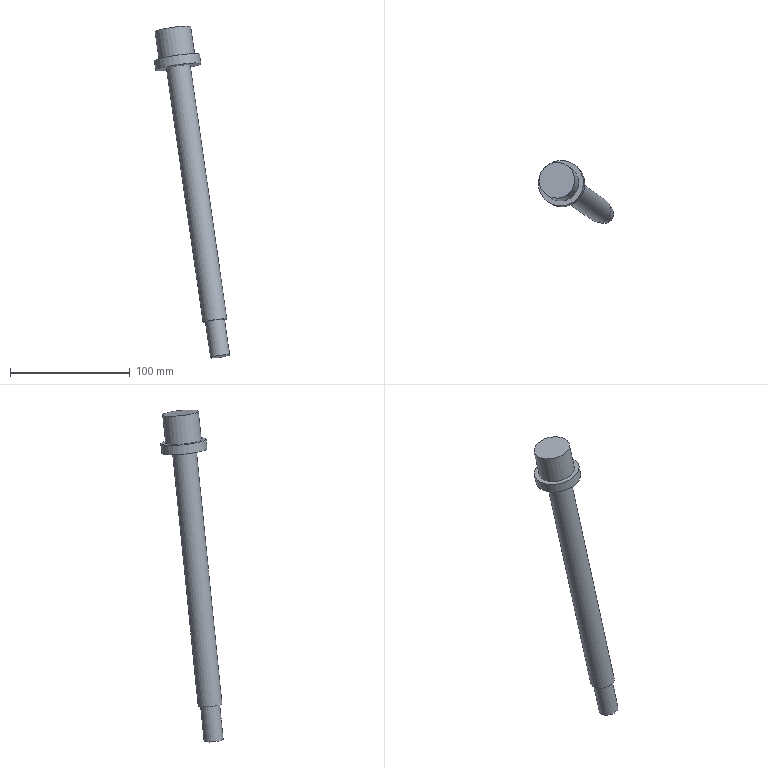Part | NX | features solid 2 | 1 solid | 9 faces | box 62.713 x 52.065 x 276.786 mm | volume 99614 mm3 | plane 5 | cylinder 4 | commonest cylinder face diameters 16 x1 20 x1 30 x1 38 x1
STEP:
#1=CARTESIAN_POINT('',(-106.68,452.312,-279.259));
#2=VERTEX_POINT('',#1);
#3=CARTESIAN_POINT('',(-110.065,461.613,-280.689));
#4=DIRECTION('',(-0.1422,0.0996,0.9848));
#5=DIRECTION('',(0.3385,-0.93,0.143));
#6=AXIS2_PLACEMENT_3D('',#3,#4,#5);
#7=CIRCLE('',#6,10.);
#8=EDGE_CURVE('',#2,#2,#7,.T.);
#9=ORIENTED_EDGE('',*,*,#8,.F.);
#10=EDGE_LOOP('',(#9));
#11=FACE_BOUND('',#10,.T.);
#12=CARTESIAN_POINT('',(-102.147,461.613,-279.545));
#13=VERTEX_POINT('',#12);
#14=CARTESIAN_POINT('',(-110.065,461.613,-280.689));
#15=DIRECTION('',(-0.1422,0.0996,0.9848));
#16=DIRECTION('',(0.9897,0.,0.143));
#17=AXIS2_PLACEMENT_3D('',#14,#15,#16);
#18=CIRCLE('',#17,8.);
#19=EDGE_CURVE('',#13,#13,#18,.F.);
#20=ORIENTED_EDGE('',*,*,#19,.F.);
#21=EDGE_LOOP('',(#20));
#22=FACE_BOUND('',#21,.T.);
#23=CARTESIAN_POINT('',(-110.065,461.613,-280.689));
#24=DIRECTION('',(-0.1422,0.0996,0.9848));
#25=DIRECTION('',(0.7628,0.645,0.04494));
#26=AXIS2_PLACEMENT_3D('',#23,#24,#25);
#27=PLANE('',#26);
#28=ADVANCED_FACE('',(#11,#22),#27,.F.);
#29=CARTESIAN_POINT('',(-127.292,496.079,-60.223));
#30=VERTEX_POINT('',#29);
#31=CARTESIAN_POINT('',(-141.786,483.823,-61.077));
#32=DIRECTION('',(-0.1422,0.0996,0.9848));
#33=DIRECTION('',(0.7628,0.645,0.04494));
#34=AXIS2_PLACEMENT_3D('',#31,#32,#33);
#35=CIRCLE('',#34,19.);
#36=EDGE_CURVE('',#30,#30,#35,.T.);
#37=ORIENTED_EDGE('',*,*,#36,.T.);
#38=EDGE_LOOP('',(#37));
#39=FACE_BOUND('',#38,.T.);
#40=CARTESIAN_POINT('',(-130.343,493.499,-60.403));
#41=VERTEX_POINT('',#40);
#42=CARTESIAN_POINT('',(-141.786,483.823,-61.077));
#43=DIRECTION('',(-0.1422,0.0996,0.9848));
#44=DIRECTION('',(0.7628,0.645,0.04494));
#45=AXIS2_PLACEMENT_3D('',#42,#43,#44);
#46=CIRCLE('',#45,15.);
#47=EDGE_CURVE('',#41,#41,#46,.T.);
#48=ORIENTED_EDGE('',*,*,#47,.F.);
#49=EDGE_LOOP('',(#48));
#50=FACE_BOUND('',#49,.T.);
#51=CARTESIAN_POINT('',(-141.786,483.823,-61.077));
#52=DIRECTION('',(-0.1422,0.0996,0.9848));
#53=DIRECTION('',(0.7628,0.645,0.04494));
#54=AXIS2_PLACEMENT_3D('',#51,#52,#53);
#55=PLANE('',#54);
#56=ADVANCED_FACE('',(#39,#50),#55,.T.);
#57=CARTESIAN_POINT('',(-137.263,473.726,-67.526));
#58=VERTEX_POINT('',#57);
#59=CARTESIAN_POINT('',(-140.648,483.027,-68.955));
#60=DIRECTION('',(-0.1422,0.0996,0.9848));
#61=DIRECTION('',(0.3385,-0.93,0.143));
#62=AXIS2_PLACEMENT_3D('',#59,#60,#61);
#63=CIRCLE('',#62,10.);
#64=EDGE_CURVE('',#58,#58,#63,.T.);
#65=ORIENTED_EDGE('',*,*,#64,.F.);
#66=EDGE_LOOP('',(#65));
#67=FACE_BOUND('',#66,.T.);
#68=ORIENTED_EDGE('',*,*,#8,.T.);
#69=EDGE_LOOP('',(#68));
#70=FACE_BOUND('',#69,.T.);
#71=CARTESIAN_POINT('',(-134.247,478.545,-113.272));
#72=DIRECTION('',(0.1422,-0.0996,-0.9848));
#73=DIRECTION('',(-0.7628,-0.645,-0.04494));
#74=AXIS2_PLACEMENT_3D('',#71,#72,#73);
#75=CYLINDRICAL_SURFACE('',#74,10.);
#76=ADVANCED_FACE('',(#67,#70),#75,.T.);
#77=CARTESIAN_POINT('',(-126.154,495.282,-68.101));
#78=VERTEX_POINT('',#77);
#79=CARTESIAN_POINT('',(-140.648,483.027,-68.955));
#80=DIRECTION('',(-0.1422,0.0996,0.9848));
#81=DIRECTION('',(0.7628,0.645,0.04494));
#82=AXIS2_PLACEMENT_3D('',#79,#80,#81);
#83=CIRCLE('',#82,19.);
#84=EDGE_CURVE('',#78,#78,#83,.T.);
#85=ORIENTED_EDGE('',*,*,#84,.F.);
#86=EDGE_LOOP('',(#85));
#87=FACE_BOUND('',#86,.T.);
#88=ORIENTED_EDGE('',*,*,#64,.T.);
#89=EDGE_LOOP('',(#88));
#90=FACE_BOUND('',#89,.T.);
#91=CARTESIAN_POINT('',(-140.648,483.027,-68.955));
#92=DIRECTION('',(-0.1422,0.0996,0.9848));
#93=DIRECTION('',(0.7628,0.645,0.04494));
#94=AXIS2_PLACEMENT_3D('',#91,#92,#93);
#95=PLANE('',#94);
#96=ADVANCED_FACE('',(#87,#90),#95,.F.);
#97=ORIENTED_EDGE('',*,*,#36,.F.);
#98=EDGE_LOOP('',(#97));
#99=FACE_BOUND('',#98,.T.);
#100=ORIENTED_EDGE('',*,*,#84,.T.);
#101=EDGE_LOOP('',(#100));
#102=FACE_BOUND('',#101,.T.);
#103=CARTESIAN_POINT('',(-141.786,483.823,-61.077));
#104=DIRECTION('',(0.1422,-0.0996,-0.9848));
#105=DIRECTION('',(-0.7628,-0.645,-0.04494));
#106=AXIS2_PLACEMENT_3D('',#103,#104,#105);
#107=CYLINDRICAL_SURFACE('',#106,19.);
#108=ADVANCED_FACE('',(#99,#102),#107,.T.);
#109=ORIENTED_EDGE('',*,*,#47,.T.);
#110=EDGE_LOOP('',(#109));
#111=FACE_BOUND('',#110,.T.);
#112=CARTESIAN_POINT('',(-133.757,495.89,-36.767));
#113=VERTEX_POINT('',#112);
#114=CARTESIAN_POINT('',(-145.2,486.214,-37.441));
#115=DIRECTION('',(-0.1422,0.0996,0.9848));
#116=DIRECTION('',(0.7628,0.645,0.04494));
#117=AXIS2_PLACEMENT_3D('',#114,#115,#116);
#118=CIRCLE('',#117,15.);
#119=EDGE_CURVE('',#113,#113,#118,.T.);
#120=ORIENTED_EDGE('',*,*,#119,.F.);
#121=EDGE_LOOP('',(#120));
#122=FACE_BOUND('',#121,.T.);
#123=CARTESIAN_POINT('',(-142.355,484.222,-57.138));
#124=DIRECTION('',(0.1422,-0.0996,-0.9848));
#125=DIRECTION('',(-0.7628,-0.645,-0.04494));
#126=AXIS2_PLACEMENT_3D('',#123,#124,#125);
#127=CYLINDRICAL_SURFACE('',#126,15.);
#128=ADVANCED_FACE('',(#111,#122),#127,.T.);
#129=ORIENTED_EDGE('',*,*,#119,.T.);
#130=EDGE_LOOP('',(#129));
#131=FACE_BOUND('',#130,.T.);
#132=CARTESIAN_POINT('',(-145.2,486.214,-37.441));
#133=DIRECTION('',(-0.1422,0.0996,0.9848));
#134=DIRECTION('',(0.7628,0.645,0.04494));
#135=AXIS2_PLACEMENT_3D('',#132,#133,#134);
#136=PLANE('',#135);
#137=ADVANCED_FACE('',(#131),#136,.T.);
#138=CARTESIAN_POINT('',(-97.88,458.625,-309.09));
#139=VERTEX_POINT('',#138);
#140=CARTESIAN_POINT('',(-105.798,458.625,-310.233));
#141=DIRECTION('',(-0.1422,0.0996,0.9848));
#142=DIRECTION('',(0.9897,0.,0.143));
#143=AXIS2_PLACEMENT_3D('',#140,#141,#142);
#144=CIRCLE('',#143,8.);
#145=EDGE_CURVE('',#139,#139,#144,.F.);
#146=ORIENTED_EDGE('',*,*,#145,.F.);
#147=EDGE_LOOP('',(#146));
#148=FACE_BOUND('',#147,.T.);
#149=ORIENTED_EDGE('',*,*,#19,.T.);
#150=EDGE_LOOP('',(#149));
#151=FACE_BOUND('',#150,.T.);
#152=CARTESIAN_POINT('',(-107.22,459.621,-300.385));
#153=DIRECTION('',(-0.1422,0.0996,0.9848));
#154=DIRECTION('',(0.9897,0.,0.143));
#155=AXIS2_PLACEMENT_3D('',#152,#153,#154);
#156=CYLINDRICAL_SURFACE('',#155,8.);
#157=ADVANCED_FACE('',(#148,#151),#156,.T.);
#158=ORIENTED_EDGE('',*,*,#145,.T.);
#159=EDGE_LOOP('',(#158));
#160=FACE_BOUND('',#159,.T.);
#161=CARTESIAN_POINT('',(-105.798,458.625,-310.233));
#162=DIRECTION('',(-0.1422,0.0996,0.9848));
#163=DIRECTION('',(-0.3452,-0.9374,0.04494));
#164=AXIS2_PLACEMENT_3D('',#161,#162,#163);
#165=PLANE('',#164);
#166=ADVANCED_FACE('',(#160),#165,.F.);
#167=CLOSED_SHELL('',(#28,#56,#76,#96,#108,#128,#137,#157,#166));
#168=MANIFOLD_SOLID_BREP('',#167);
#169=(LENGTH_UNIT()NAMED_UNIT(*)SI_UNIT(.MILLI.,.METRE.));
#170=UNCERTAINTY_MEASURE_WITH_UNIT(LENGTH_MEASURE(0.00001),#169,'','');
#171=(NAMED_UNIT(*)PLANE_ANGLE_UNIT()SI_UNIT($,.RADIAN.));
#172=(NAMED_UNIT(*)SI_UNIT($,.STERADIAN.)SOLID_ANGLE_UNIT());
#173=(GEOMETRIC_REPRESENTATION_CONTEXT(3)GLOBAL_UNCERTAINTY_ASSIGNED_CONTEXT((#170))GLOBAL_UNIT_ASSIGNED_CONTEXT((#169,#171,#172))REPRESENTATION_CONTEXT('',''));
#174=ADVANCED_BREP_SHAPE_REPRESENTATION('',(#168),#173);